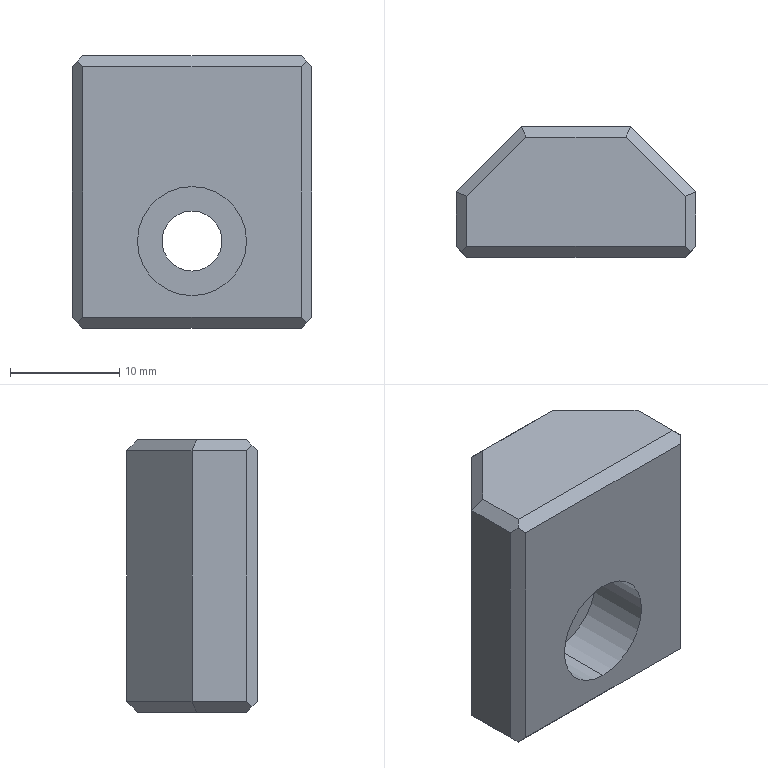Part | Creo | 1 solid | 27 faces | box 22 x 12 x 25 mm | volume 5004 mm3 | plane 23 | cylinder 4 | commonest cylinder face diameters 5.5 x2 10 x2
STEP:
#1=CARTESIAN_POINT('',(34.742,-375.005,-60.5));
#2=VERTEX_POINT('',#1);
#3=CARTESIAN_POINT('',(34.742,-375.005,-70.5));
#4=VERTEX_POINT('',#3);
#5=CARTESIAN_POINT('',(34.742,-375.005,-65.5));
#6=DIRECTION('',(0.,1.,0.));
#7=DIRECTION('',(0.,0.,1.));
#8=AXIS2_PLACEMENT_3D('',#5,#6,#7);
#9=CIRCLE('',#8,5.);
#10=EDGE_CURVE('',#2,#4,#9,.T.);
#11=ORIENTED_EDGE('',*,*,#10,.T.);
#12=CARTESIAN_POINT('',(34.742,-369.005,-70.5));
#13=VERTEX_POINT('',#12);
#14=CARTESIAN_POINT('',(34.742,-375.005,-70.5));
#15=DIRECTION('',(0.,1.,0.));
#16=VECTOR('',#15,6.);
#17=LINE('',#14,#16);
#18=EDGE_CURVE('',#4,#13,#17,.T.);
#19=ORIENTED_EDGE('',*,*,#18,.T.);
#20=CARTESIAN_POINT('',(34.742,-369.005,-60.5));
#21=VERTEX_POINT('',#20);
#22=CARTESIAN_POINT('',(34.742,-369.005,-65.5));
#23=DIRECTION('',(0.,-1.,0.));
#24=DIRECTION('',(0.,0.,-1.));
#25=AXIS2_PLACEMENT_3D('',#22,#23,#24);
#26=CIRCLE('',#25,5.);
#27=EDGE_CURVE('',#13,#21,#26,.T.);
#28=ORIENTED_EDGE('',*,*,#27,.T.);
#29=CARTESIAN_POINT('',(34.742,-375.005,-60.5));
#30=DIRECTION('',(0.,1.,0.));
#31=VECTOR('',#30,6.);
#32=LINE('',#29,#31);
#33=EDGE_CURVE('',#2,#21,#32,.T.);
#34=ORIENTED_EDGE('',*,*,#33,.F.);
#35=EDGE_LOOP('',(#11,#19,#28,#34));
#36=FACE_OUTER_BOUND('',#35,.F.);
#37=CARTESIAN_POINT('',(34.742,-375.305,-65.5));
#38=DIRECTION('',(0.,1.,0.));
#39=DIRECTION('',(0.,0.,1.));
#40=AXIS2_PLACEMENT_3D('',#37,#38,#39);
#41=CYLINDRICAL_SURFACE('',#40,5.);
#42=ADVANCED_FACE('',(#36),#41,.F.);
#43=CARTESIAN_POINT('',(44.742,-375.005,-72.5));
#44=VERTEX_POINT('',#43);
#45=CARTESIAN_POINT('',(44.742,-375.005,-49.5));
#46=VERTEX_POINT('',#45);
#47=CARTESIAN_POINT('',(44.742,-375.005,-72.5));
#48=DIRECTION('',(0.,0.,1.));
#49=VECTOR('',#48,23.);
#50=LINE('',#47,#49);
#51=EDGE_CURVE('',#44,#46,#50,.T.);
#52=ORIENTED_EDGE('',*,*,#51,.F.);
#53=CARTESIAN_POINT('',(24.742,-375.005,-72.5));
#54=VERTEX_POINT('',#53);
#55=CARTESIAN_POINT('',(44.742,-375.005,-72.5));
#56=DIRECTION('',(-1.,0.,0.));
#57=VECTOR('',#56,20.);
#58=LINE('',#55,#57);
#59=EDGE_CURVE('',#44,#54,#58,.T.);
#60=ORIENTED_EDGE('',*,*,#59,.T.);
#61=CARTESIAN_POINT('',(24.742,-375.005,-49.5));
#62=VERTEX_POINT('',#61);
#63=CARTESIAN_POINT('',(24.742,-375.005,-49.5));
#64=DIRECTION('',(0.,0.,-1.));
#65=VECTOR('',#64,23.);
#66=LINE('',#63,#65);
#67=EDGE_CURVE('',#62,#54,#66,.T.);
#68=ORIENTED_EDGE('',*,*,#67,.F.);
#69=CARTESIAN_POINT('',(44.742,-375.005,-49.5));
#70=DIRECTION('',(-1.,0.,0.));
#71=VECTOR('',#70,20.);
#72=LINE('',#69,#71);
#73=EDGE_CURVE('',#46,#62,#72,.T.);
#74=ORIENTED_EDGE('',*,*,#73,.F.);
#75=EDGE_LOOP('',(#52,#60,#68,#74));
#76=FACE_OUTER_BOUND('',#75,.F.);
#77=CARTESIAN_POINT('',(34.742,-375.005,-65.5));
#78=DIRECTION('',(0.,1.,0.));
#79=DIRECTION('',(0.,0.,-1.));
#80=AXIS2_PLACEMENT_3D('',#77,#78,#79);
#81=CIRCLE('',#80,5.);
#82=EDGE_CURVE('',#4,#2,#81,.T.);
#83=ORIENTED_EDGE('',*,*,#82,.F.);
#84=ORIENTED_EDGE('',*,*,#10,.F.);
#85=EDGE_LOOP('',(#83,#84));
#86=FACE_BOUND('',#85,.F.);
#87=CARTESIAN_POINT('',(45.742,-375.005,-73.5));
#88=DIRECTION('',(0.,-1.,0.));
#89=DIRECTION('',(0.,0.,-1.));
#90=AXIS2_PLACEMENT_3D('',#87,#88,#89);
#91=PLANE('',#90);
#92=ADVANCED_FACE('',(#76,#86),#91,.T.);
#93=ORIENTED_EDGE('',*,*,#82,.T.);
#94=ORIENTED_EDGE('',*,*,#33,.T.);
#95=CARTESIAN_POINT('',(34.742,-369.005,-65.5));
#96=DIRECTION('',(0.,-1.,0.));
#97=DIRECTION('',(0.,0.,1.));
#98=AXIS2_PLACEMENT_3D('',#95,#96,#97);
#99=CIRCLE('',#98,5.);
#100=EDGE_CURVE('',#21,#13,#99,.T.);
#101=ORIENTED_EDGE('',*,*,#100,.T.);
#102=ORIENTED_EDGE('',*,*,#18,.F.);
#103=EDGE_LOOP('',(#93,#94,#101,#102));
#104=FACE_OUTER_BOUND('',#103,.F.);
#105=CARTESIAN_POINT('',(34.742,-375.305,-65.5));
#106=DIRECTION('',(0.,1.,0.));
#107=DIRECTION('',(0.,0.,1.));
#108=AXIS2_PLACEMENT_3D('',#105,#106,#107);
#109=CYLINDRICAL_SURFACE('',#108,5.);
#110=ADVANCED_FACE('',(#104),#109,.F.);
#111=ORIENTED_EDGE('',*,*,#27,.F.);
#112=ORIENTED_EDGE('',*,*,#100,.F.);
#113=EDGE_LOOP('',(#111,#112));
#114=FACE_OUTER_BOUND('',#113,.F.);
#115=CARTESIAN_POINT('',(34.742,-369.005,-68.25));
#116=VERTEX_POINT('',#115);
#117=CARTESIAN_POINT('',(34.742,-369.005,-62.75));
#118=VERTEX_POINT('',#117);
#119=CARTESIAN_POINT('',(34.742,-369.005,-65.5));
#120=DIRECTION('',(0.,1.,0.));
#121=DIRECTION('',(0.,0.,-1.));
#122=AXIS2_PLACEMENT_3D('',#119,#120,#121);
#123=CIRCLE('',#122,2.75);
#124=EDGE_CURVE('',#116,#118,#123,.T.);
#125=ORIENTED_EDGE('',*,*,#124,.F.);
#126=CARTESIAN_POINT('',(34.742,-369.005,-65.5));
#127=DIRECTION('',(0.,1.,0.));
#128=DIRECTION('',(0.,0.,1.));
#129=AXIS2_PLACEMENT_3D('',#126,#127,#128);
#130=CIRCLE('',#129,2.75);
#131=EDGE_CURVE('',#118,#116,#130,.T.);
#132=ORIENTED_EDGE('',*,*,#131,.F.);
#133=EDGE_LOOP('',(#125,#132));
#134=FACE_BOUND('',#133,.F.);
#135=CARTESIAN_POINT('',(34.742,-369.005,-65.5));
#136=DIRECTION('',(0.,1.,0.));
#137=DIRECTION('',(0.,0.,1.));
#138=AXIS2_PLACEMENT_3D('',#135,#136,#137);
#139=PLANE('',#138);
#140=ADVANCED_FACE('',(#114,#134),#139,.F.);
#141=CARTESIAN_POINT('',(34.742,-363.005,-62.75));
#142=VERTEX_POINT('',#141);
#143=CARTESIAN_POINT('',(34.742,-363.005,-68.25));
#144=VERTEX_POINT('',#143);
#145=CARTESIAN_POINT('',(34.742,-363.005,-65.5));
#146=DIRECTION('',(0.,-1.,0.));
#147=DIRECTION('',(0.,0.,1.));
#148=AXIS2_PLACEMENT_3D('',#145,#146,#147);
#149=CIRCLE('',#148,2.75);
#150=EDGE_CURVE('',#142,#144,#149,.T.);
#151=ORIENTED_EDGE('',*,*,#150,.T.);
#152=CARTESIAN_POINT('',(34.742,-363.005,-68.25));
#153=DIRECTION('',(0.,-1.,0.));
#154=VECTOR('',#153,6.);
#155=LINE('',#152,#154);
#156=EDGE_CURVE('',#144,#116,#155,.T.);
#157=ORIENTED_EDGE('',*,*,#156,.T.);
#158=ORIENTED_EDGE('',*,*,#124,.T.);
#159=CARTESIAN_POINT('',(34.742,-363.005,-62.75));
#160=DIRECTION('',(0.,-1.,0.));
#161=VECTOR('',#160,6.);
#162=LINE('',#159,#161);
#163=EDGE_CURVE('',#142,#118,#162,.T.);
#164=ORIENTED_EDGE('',*,*,#163,.F.);
#165=EDGE_LOOP('',(#151,#157,#158,#164));
#166=FACE_OUTER_BOUND('',#165,.F.);
#167=CARTESIAN_POINT('',(34.742,-369.005,-65.5));
#168=DIRECTION('',(0.,-1.,0.));
#169=DIRECTION('',(0.,0.,1.));
#170=AXIS2_PLACEMENT_3D('',#167,#168,#169);
#171=CYLINDRICAL_SURFACE('',#170,2.75);
#172=ADVANCED_FACE('',(#166),#171,.F.);
#173=CARTESIAN_POINT('',(29.742,-363.005,-72.5));
#174=VERTEX_POINT('',#173);
#175=CARTESIAN_POINT('',(29.742,-363.005,-49.5));
#176=VERTEX_POINT('',#175);
#177=CARTESIAN_POINT('',(29.742,-363.005,-72.5));
#178=DIRECTION('',(0.,0.,1.));
#179=VECTOR('',#178,23.);
#180=LINE('',#177,#179);
#181=EDGE_CURVE('',#174,#176,#180,.T.);
#182=ORIENTED_EDGE('',*,*,#181,.F.);
#183=CARTESIAN_POINT('',(39.742,-363.005,-72.5));
#184=VERTEX_POINT('',#183);
#185=CARTESIAN_POINT('',(39.742,-363.005,-72.5));
#186=DIRECTION('',(-1.,0.,0.));
#187=VECTOR('',#186,10.);
#188=LINE('',#185,#187);
#189=EDGE_CURVE('',#184,#174,#188,.T.);
#190=ORIENTED_EDGE('',*,*,#189,.F.);
#191=CARTESIAN_POINT('',(39.742,-363.005,-49.5));
#192=VERTEX_POINT('',#191);
#193=CARTESIAN_POINT('',(39.742,-363.005,-49.5));
#194=DIRECTION('',(0.,0.,-1.));
#195=VECTOR('',#194,23.);
#196=LINE('',#193,#195);
#197=EDGE_CURVE('',#192,#184,#196,.T.);
#198=ORIENTED_EDGE('',*,*,#197,.F.);
#199=CARTESIAN_POINT('',(39.742,-363.005,-49.5));
#200=DIRECTION('',(-1.,0.,0.));
#201=VECTOR('',#200,10.);
#202=LINE('',#199,#201);
#203=EDGE_CURVE('',#192,#176,#202,.T.);
#204=ORIENTED_EDGE('',*,*,#203,.T.);
#205=EDGE_LOOP('',(#182,#190,#198,#204));
#206=FACE_OUTER_BOUND('',#205,.F.);
#207=CARTESIAN_POINT('',(34.742,-363.005,-65.5));
#208=DIRECTION('',(0.,-1.,0.));
#209=DIRECTION('',(0.,0.,-1.));
#210=AXIS2_PLACEMENT_3D('',#207,#208,#209);
#211=CIRCLE('',#210,2.75);
#212=EDGE_CURVE('',#144,#142,#211,.T.);
#213=ORIENTED_EDGE('',*,*,#212,.F.);
#214=ORIENTED_EDGE('',*,*,#150,.F.);
#215=EDGE_LOOP('',(#213,#214));
#216=FACE_BOUND('',#215,.F.);
#217=CARTESIAN_POINT('',(45.742,-363.005,-48.5));
#218=DIRECTION('',(0.,1.,0.));
#219=DIRECTION('',(0.,0.,1.));
#220=AXIS2_PLACEMENT_3D('',#217,#218,#219);
#221=PLANE('',#220);
#222=ADVANCED_FACE('',(#206,#216),#221,.T.);
#223=ORIENTED_EDGE('',*,*,#212,.T.);
#224=ORIENTED_EDGE('',*,*,#163,.T.);
#225=ORIENTED_EDGE('',*,*,#131,.T.);
#226=ORIENTED_EDGE('',*,*,#156,.F.);
#227=EDGE_LOOP('',(#223,#224,#225,#226));
#228=FACE_OUTER_BOUND('',#227,.F.);
#229=CARTESIAN_POINT('',(34.742,-369.005,-65.5));
#230=DIRECTION('',(0.,-1.,0.));
#231=DIRECTION('',(0.,0.,1.));
#232=AXIS2_PLACEMENT_3D('',#229,#230,#231);
#233=CYLINDRICAL_SURFACE('',#232,2.75);
#234=ADVANCED_FACE('',(#228),#233,.F.);
#235=CARTESIAN_POINT('',(23.742,-369.005,-72.5));
#236=VERTEX_POINT('',#235);
#237=CARTESIAN_POINT('',(23.742,-369.005,-49.5));
#238=VERTEX_POINT('',#237);
#239=CARTESIAN_POINT('',(23.742,-369.005,-72.5));
#240=DIRECTION('',(0.,0.,1.));
#241=VECTOR('',#240,23.);
#242=LINE('',#239,#241);
#243=EDGE_CURVE('',#236,#238,#242,.T.);
#244=ORIENTED_EDGE('',*,*,#243,.F.);
#245=CARTESIAN_POINT('',(29.742,-363.005,-72.5));
#246=DIRECTION('',(-0.7071,-0.7071,0.));
#247=VECTOR('',#246,8.485);
#248=LINE('',#245,#247);
#249=EDGE_CURVE('',#174,#236,#248,.T.);
#250=ORIENTED_EDGE('',*,*,#249,.F.);
#251=ORIENTED_EDGE('',*,*,#181,.T.);
#252=CARTESIAN_POINT('',(23.742,-369.005,-49.5));
#253=DIRECTION('',(0.7071,0.7071,0.));
#254=VECTOR('',#253,8.485);
#255=LINE('',#252,#254);
#256=EDGE_CURVE('',#238,#176,#255,.T.);
#257=ORIENTED_EDGE('',*,*,#256,.F.);
#258=EDGE_LOOP('',(#244,#250,#251,#257));
#259=FACE_OUTER_BOUND('',#258,.F.);
#260=CARTESIAN_POINT('',(26.742,-366.005,-61.));
#261=DIRECTION('',(-0.7071,0.7071,0.));
#262=DIRECTION('',(0.,0.,1.));
#263=AXIS2_PLACEMENT_3D('',#260,#261,#262);
#264=PLANE('',#263);
#265=ADVANCED_FACE('',(#259),#264,.T.);
#266=CARTESIAN_POINT('',(23.742,-374.005,-49.5));
#267=VERTEX_POINT('',#266);
#268=CARTESIAN_POINT('',(23.742,-374.005,-72.5));
#269=VERTEX_POINT('',#268);
#270=CARTESIAN_POINT('',(23.742,-374.005,-49.5));
#271=DIRECTION('',(0.,0.,-1.));
#272=VECTOR('',#271,23.);
#273=LINE('',#270,#272);
#274=EDGE_CURVE('',#267,#269,#273,.T.);
#275=ORIENTED_EDGE('',*,*,#274,.T.);
#276=CARTESIAN_POINT('',(23.742,-374.005,-72.5));
#277=DIRECTION('',(0.,1.,0.));
#278=VECTOR('',#277,5.);
#279=LINE('',#276,#278);
#280=EDGE_CURVE('',#269,#236,#279,.T.);
#281=ORIENTED_EDGE('',*,*,#280,.T.);
#282=ORIENTED_EDGE('',*,*,#243,.T.);
#283=CARTESIAN_POINT('',(23.742,-369.005,-49.5));
#284=DIRECTION('',(0.,-1.,0.));
#285=VECTOR('',#284,5.);
#286=LINE('',#283,#285);
#287=EDGE_CURVE('',#238,#267,#286,.T.);
#288=ORIENTED_EDGE('',*,*,#287,.T.);
#289=EDGE_LOOP('',(#275,#281,#282,#288));
#290=FACE_OUTER_BOUND('',#289,.F.);
#291=CARTESIAN_POINT('',(23.742,-375.005,-53.5));
#292=DIRECTION('',(-1.,0.,0.));
#293=DIRECTION('',(0.,1.,0.));
#294=AXIS2_PLACEMENT_3D('',#291,#292,#293);
#295=PLANE('',#294);
#296=ADVANCED_FACE('',(#290),#295,.T.);
#297=CARTESIAN_POINT('',(24.242,-374.505,-49.));
#298=VERTEX_POINT('',#297);
#299=CARTESIAN_POINT('',(24.742,-375.005,-49.5));
#300=DIRECTION('',(-0.5774,0.5774,0.5774));
#301=VECTOR('',#300,0.866);
#302=LINE('',#299,#301);
#303=EDGE_CURVE('',#62,#298,#302,.T.);
#304=ORIENTED_EDGE('',*,*,#303,.F.);
#305=ORIENTED_EDGE('',*,*,#67,.T.);
#306=CARTESIAN_POINT('',(24.242,-374.505,-73.));
#307=VERTEX_POINT('',#306);
#308=CARTESIAN_POINT('',(24.242,-374.505,-73.));
#309=DIRECTION('',(0.5774,-0.5774,0.5774));
#310=VECTOR('',#309,0.866);
#311=LINE('',#308,#310);
#312=EDGE_CURVE('',#307,#54,#311,.T.);
#313=ORIENTED_EDGE('',*,*,#312,.F.);
#314=CARTESIAN_POINT('',(23.742,-374.005,-72.5));
#315=DIRECTION('',(0.5774,-0.5774,-0.5774));
#316=VECTOR('',#315,0.866);
#317=LINE('',#314,#316);
#318=EDGE_CURVE('',#269,#307,#317,.T.);
#319=ORIENTED_EDGE('',*,*,#318,.F.);
#320=ORIENTED_EDGE('',*,*,#274,.F.);
#321=CARTESIAN_POINT('',(24.242,-374.505,-49.));
#322=DIRECTION('',(-0.5774,0.5774,-0.5774));
#323=VECTOR('',#322,0.866);
#324=LINE('',#321,#323);
#325=EDGE_CURVE('',#298,#267,#324,.T.);
#326=ORIENTED_EDGE('',*,*,#325,.F.);
#327=EDGE_LOOP('',(#304,#305,#313,#319,#320,#326));
#328=FACE_OUTER_BOUND('',#327,.F.);
#329=CARTESIAN_POINT('',(24.242,-374.505,-61.));
#330=DIRECTION('',(-0.7071,-0.7071,0.));
#331=DIRECTION('',(-0.7071,0.7071,0.));
#332=AXIS2_PLACEMENT_3D('',#329,#330,#331);
#333=PLANE('',#332);
#334=ADVANCED_FACE('',(#328),#333,.T.);
#335=CARTESIAN_POINT('',(24.742,-374.005,-48.5));
#336=VERTEX_POINT('',#335);
#337=CARTESIAN_POINT('',(24.242,-374.505,-49.));
#338=DIRECTION('',(0.5774,0.5774,0.5774));
#339=VECTOR('',#338,0.866);
#340=LINE('',#337,#339);
#341=EDGE_CURVE('',#298,#336,#340,.T.);
#342=ORIENTED_EDGE('',*,*,#341,.T.);
#343=CARTESIAN_POINT('',(44.742,-374.005,-48.5));
#344=VERTEX_POINT('',#343);
#345=CARTESIAN_POINT('',(44.742,-374.005,-48.5));
#346=DIRECTION('',(-1.,0.,0.));
#347=VECTOR('',#346,20.);
#348=LINE('',#345,#347);
#349=EDGE_CURVE('',#344,#336,#348,.T.);
#350=ORIENTED_EDGE('',*,*,#349,.F.);
#351=CARTESIAN_POINT('',(45.242,-374.505,-49.));
#352=VERTEX_POINT('',#351);
#353=CARTESIAN_POINT('',(45.242,-374.505,-49.));
#354=DIRECTION('',(-0.5774,0.5774,0.5774));
#355=VECTOR('',#354,0.866);
#356=LINE('',#353,#355);
#357=EDGE_CURVE('',#352,#344,#356,.T.);
#358=ORIENTED_EDGE('',*,*,#357,.F.);
#359=CARTESIAN_POINT('',(45.242,-374.505,-49.));
#360=DIRECTION('',(-0.5774,-0.5774,-0.5774));
#361=VECTOR('',#360,0.866);
#362=LINE('',#359,#361);
#363=EDGE_CURVE('',#352,#46,#362,.T.);
#364=ORIENTED_EDGE('',*,*,#363,.T.);
#365=ORIENTED_EDGE('',*,*,#73,.T.);
#366=ORIENTED_EDGE('',*,*,#303,.T.);
#367=EDGE_LOOP('',(#342,#350,#358,#364,#365,#366));
#368=FACE_OUTER_BOUND('',#367,.F.);
#369=CARTESIAN_POINT('',(34.742,-374.505,-49.));
#370=DIRECTION('',(0.,-0.7071,0.7071));
#371=DIRECTION('',(0.,0.7071,0.7071));
#372=AXIS2_PLACEMENT_3D('',#369,#370,#371);
#373=PLANE('',#372);
#374=ADVANCED_FACE('',(#368),#373,.T.);
#375=CARTESIAN_POINT('',(24.742,-369.419,-48.5));
#376=VERTEX_POINT('',#375);
#377=CARTESIAN_POINT('',(24.742,-369.419,-48.5));
#378=DIRECTION('',(-0.6786,0.2811,-0.6786));
#379=VECTOR('',#378,1.474);
#380=LINE('',#377,#379);
#381=EDGE_CURVE('',#376,#238,#380,.T.);
#382=ORIENTED_EDGE('',*,*,#381,.F.);
#383=CARTESIAN_POINT('',(24.742,-369.419,-48.5));
#384=DIRECTION('',(0.,-1.,0.));
#385=VECTOR('',#384,4.586);
#386=LINE('',#383,#385);
#387=EDGE_CURVE('',#376,#336,#386,.T.);
#388=ORIENTED_EDGE('',*,*,#387,.T.);
#389=ORIENTED_EDGE('',*,*,#341,.F.);
#390=ORIENTED_EDGE('',*,*,#325,.T.);
#391=ORIENTED_EDGE('',*,*,#287,.F.);
#392=EDGE_LOOP('',(#382,#388,#389,#390,#391));
#393=FACE_OUTER_BOUND('',#392,.F.);
#394=CARTESIAN_POINT('',(24.242,-372.005,-49.));
#395=DIRECTION('',(-0.7071,0.,0.7071));
#396=DIRECTION('',(-0.7071,0.,-0.7071));
#397=AXIS2_PLACEMENT_3D('',#394,#395,#396);
#398=PLANE('',#397);
#399=ADVANCED_FACE('',(#393),#398,.T.);
#400=CARTESIAN_POINT('',(30.156,-364.005,-48.5));
#401=VERTEX_POINT('',#400);
#402=CARTESIAN_POINT('',(30.156,-364.005,-48.5));
#403=DIRECTION('',(-0.2811,0.6786,-0.6786));
#404=VECTOR('',#403,1.474);
#405=LINE('',#402,#404);
#406=EDGE_CURVE('',#401,#176,#405,.T.);
#407=ORIENTED_EDGE('',*,*,#406,.F.);
#408=CARTESIAN_POINT('',(30.156,-364.005,-48.5));
#409=DIRECTION('',(-0.7071,-0.7071,0.));
#410=VECTOR('',#409,7.657);
#411=LINE('',#408,#410);
#412=EDGE_CURVE('',#401,#376,#411,.T.);
#413=ORIENTED_EDGE('',*,*,#412,.T.);
#414=ORIENTED_EDGE('',*,*,#381,.T.);
#415=ORIENTED_EDGE('',*,*,#256,.T.);
#416=EDGE_LOOP('',(#407,#413,#414,#415));
#417=FACE_OUTER_BOUND('',#416,.F.);
#418=CARTESIAN_POINT('',(27.095,-366.358,-49.));
#419=DIRECTION('',(-0.5,0.5,0.7071));
#420=DIRECTION('',(0.5,-0.5,0.7071));
#421=AXIS2_PLACEMENT_3D('',#418,#419,#420);
#422=PLANE('',#421);
#423=ADVANCED_FACE('',(#417),#422,.T.);
#424=CARTESIAN_POINT('',(39.327,-364.005,-48.5));
#425=VERTEX_POINT('',#424);
#426=CARTESIAN_POINT('',(39.327,-364.005,-48.5));
#427=DIRECTION('',(0.2811,0.6786,-0.6786));
#428=VECTOR('',#427,1.474);
#429=LINE('',#426,#428);
#430=EDGE_CURVE('',#425,#192,#429,.T.);
#431=ORIENTED_EDGE('',*,*,#430,.F.);
#432=CARTESIAN_POINT('',(39.327,-364.005,-48.5));
#433=DIRECTION('',(-1.,0.,0.));
#434=VECTOR('',#433,9.172);
#435=LINE('',#432,#434);
#436=EDGE_CURVE('',#425,#401,#435,.T.);
#437=ORIENTED_EDGE('',*,*,#436,.T.);
#438=ORIENTED_EDGE('',*,*,#406,.T.);
#439=ORIENTED_EDGE('',*,*,#203,.F.);
#440=EDGE_LOOP('',(#431,#437,#438,#439));
#441=FACE_OUTER_BOUND('',#440,.F.);
#442=CARTESIAN_POINT('',(34.742,-363.505,-49.));
#443=DIRECTION('',(0.,0.7071,0.7071));
#444=DIRECTION('',(0.,0.7071,-0.7071));
#445=AXIS2_PLACEMENT_3D('',#442,#443,#444);
#446=PLANE('',#445);
#447=ADVANCED_FACE('',(#441),#446,.T.);
#448=ORIENTED_EDGE('',*,*,#430,.T.);
#449=CARTESIAN_POINT('',(45.742,-369.005,-49.5));
#450=VERTEX_POINT('',#449);
#451=CARTESIAN_POINT('',(39.742,-363.005,-49.5));
#452=DIRECTION('',(0.7071,-0.7071,0.));
#453=VECTOR('',#452,8.485);
#454=LINE('',#451,#453);
#455=EDGE_CURVE('',#192,#450,#454,.T.);
#456=ORIENTED_EDGE('',*,*,#455,.T.);
#457=CARTESIAN_POINT('',(44.742,-369.419,-48.5));
#458=VERTEX_POINT('',#457);
#459=CARTESIAN_POINT('',(45.742,-369.005,-49.5));
#460=DIRECTION('',(-0.6786,-0.2811,0.6786));
#461=VECTOR('',#460,1.474);
#462=LINE('',#459,#461);
#463=EDGE_CURVE('',#450,#458,#462,.T.);
#464=ORIENTED_EDGE('',*,*,#463,.T.);
#465=CARTESIAN_POINT('',(44.742,-369.419,-48.5));
#466=DIRECTION('',(-0.7071,0.7071,0.));
#467=VECTOR('',#466,7.657);
#468=LINE('',#465,#467);
#469=EDGE_CURVE('',#458,#425,#468,.T.);
#470=ORIENTED_EDGE('',*,*,#469,.T.);
#471=EDGE_LOOP('',(#448,#456,#464,#470));
#472=FACE_OUTER_BOUND('',#471,.F.);
#473=CARTESIAN_POINT('',(42.388,-366.358,-49.));
#474=DIRECTION('',(0.5,0.5,0.7071));
#475=DIRECTION('',(-0.5,-0.5,0.7071));
#476=AXIS2_PLACEMENT_3D('',#473,#474,#475);
#477=PLANE('',#476);
#478=ADVANCED_FACE('',(#472),#477,.T.);
#479=ORIENTED_EDGE('',*,*,#197,.T.);
#480=CARTESIAN_POINT('',(45.742,-369.005,-72.5));
#481=VERTEX_POINT('',#480);
#482=CARTESIAN_POINT('',(45.742,-369.005,-72.5));
#483=DIRECTION('',(-0.7071,0.7071,0.));
#484=VECTOR('',#483,8.485);
#485=LINE('',#482,#484);
#486=EDGE_CURVE('',#481,#184,#485,.T.);
#487=ORIENTED_EDGE('',*,*,#486,.F.);
#488=CARTESIAN_POINT('',(45.742,-369.005,-49.5));
#489=DIRECTION('',(0.,0.,-1.));
#490=VECTOR('',#489,23.);
#491=LINE('',#488,#490);
#492=EDGE_CURVE('',#450,#481,#491,.T.);
#493=ORIENTED_EDGE('',*,*,#492,.F.);
#494=ORIENTED_EDGE('',*,*,#455,.F.);
#495=EDGE_LOOP('',(#479,#487,#493,#494));
#496=FACE_OUTER_BOUND('',#495,.F.);
#497=CARTESIAN_POINT('',(42.742,-366.005,-61.));
#498=DIRECTION('',(0.7071,0.7071,0.));
#499=DIRECTION('',(0.,0.,1.));
#500=AXIS2_PLACEMENT_3D('',#497,#498,#499);
#501=PLANE('',#500);
#502=ADVANCED_FACE('',(#496),#501,.T.);
#503=CARTESIAN_POINT('',(44.742,-369.419,-73.5));
#504=VERTEX_POINT('',#503);
#505=CARTESIAN_POINT('',(45.742,-369.005,-72.5));
#506=DIRECTION('',(-0.6786,-0.2811,-0.6786));
#507=VECTOR('',#506,1.474);
#508=LINE('',#505,#507);
#509=EDGE_CURVE('',#481,#504,#508,.T.);
#510=ORIENTED_EDGE('',*,*,#509,.F.);
#511=ORIENTED_EDGE('',*,*,#486,.T.);
#512=CARTESIAN_POINT('',(39.327,-364.005,-73.5));
#513=VERTEX_POINT('',#512);
#514=CARTESIAN_POINT('',(39.742,-363.005,-72.5));
#515=DIRECTION('',(-0.2811,-0.6786,-0.6786));
#516=VECTOR('',#515,1.474);
#517=LINE('',#514,#516);
#518=EDGE_CURVE('',#184,#513,#517,.T.);
#519=ORIENTED_EDGE('',*,*,#518,.T.);
#520=CARTESIAN_POINT('',(39.327,-364.005,-73.5));
#521=DIRECTION('',(0.7071,-0.7071,0.));
#522=VECTOR('',#521,7.657);
#523=LINE('',#520,#522);
#524=EDGE_CURVE('',#513,#504,#523,.T.);
#525=ORIENTED_EDGE('',*,*,#524,.T.);
#526=EDGE_LOOP('',(#510,#511,#519,#525));
#527=FACE_OUTER_BOUND('',#526,.F.);
#528=CARTESIAN_POINT('',(42.388,-366.358,-73.));
#529=DIRECTION('',(0.5,0.5,-0.7071));
#530=DIRECTION('',(-0.5,-0.5,-0.7071));
#531=AXIS2_PLACEMENT_3D('',#528,#529,#530);
#532=PLANE('',#531);
#533=ADVANCED_FACE('',(#527),#532,.T.);
#534=ORIENTED_EDGE('',*,*,#509,.T.);
#535=CARTESIAN_POINT('',(44.742,-374.005,-73.5));
#536=VERTEX_POINT('',#535);
#537=CARTESIAN_POINT('',(44.742,-369.419,-73.5));
#538=DIRECTION('',(0.,-1.,0.));
#539=VECTOR('',#538,4.586);
#540=LINE('',#537,#539);
#541=EDGE_CURVE('',#504,#536,#540,.T.);
#542=ORIENTED_EDGE('',*,*,#541,.T.);
#543=CARTESIAN_POINT('',(45.242,-374.505,-73.));
#544=VERTEX_POINT('',#543);
#545=CARTESIAN_POINT('',(45.242,-374.505,-73.));
#546=DIRECTION('',(-0.5774,0.5774,-0.5774));
#547=VECTOR('',#546,0.866);
#548=LINE('',#545,#547);
#549=EDGE_CURVE('',#544,#536,#548,.T.);
#550=ORIENTED_EDGE('',*,*,#549,.F.);
#551=CARTESIAN_POINT('',(45.742,-374.005,-72.5));
#552=VERTEX_POINT('',#551);
#553=CARTESIAN_POINT('',(45.242,-374.505,-73.));
#554=DIRECTION('',(0.5774,0.5774,0.5774));
#555=VECTOR('',#554,0.866);
#556=LINE('',#553,#555);
#557=EDGE_CURVE('',#544,#552,#556,.T.);
#558=ORIENTED_EDGE('',*,*,#557,.T.);
#559=CARTESIAN_POINT('',(45.742,-369.005,-72.5));
#560=DIRECTION('',(0.,-1.,0.));
#561=VECTOR('',#560,5.);
#562=LINE('',#559,#561);
#563=EDGE_CURVE('',#481,#552,#562,.T.);
#564=ORIENTED_EDGE('',*,*,#563,.F.);
#565=EDGE_LOOP('',(#534,#542,#550,#558,#564));
#566=FACE_OUTER_BOUND('',#565,.F.);
#567=CARTESIAN_POINT('',(45.242,-372.005,-73.));
#568=DIRECTION('',(0.7071,0.,-0.7071));
#569=DIRECTION('',(0.7071,0.,0.7071));
#570=AXIS2_PLACEMENT_3D('',#567,#568,#569);
#571=PLANE('',#570);
#572=ADVANCED_FACE('',(#566),#571,.T.);
#573=CARTESIAN_POINT('',(24.742,-374.005,-73.5));
#574=VERTEX_POINT('',#573);
#575=CARTESIAN_POINT('',(24.742,-369.419,-73.5));
#576=VERTEX_POINT('',#575);
#577=CARTESIAN_POINT('',(24.742,-374.005,-73.5));
#578=DIRECTION('',(0.,1.,0.));
#579=VECTOR('',#578,4.586);
#580=LINE('',#577,#579);
#581=EDGE_CURVE('',#574,#576,#580,.T.);
#582=ORIENTED_EDGE('',*,*,#581,.F.);
#583=CARTESIAN_POINT('',(44.742,-374.005,-73.5));
#584=DIRECTION('',(-1.,0.,0.));
#585=VECTOR('',#584,20.);
#586=LINE('',#583,#585);
#587=EDGE_CURVE('',#536,#574,#586,.T.);
#588=ORIENTED_EDGE('',*,*,#587,.F.);
#589=ORIENTED_EDGE('',*,*,#541,.F.);
#590=ORIENTED_EDGE('',*,*,#524,.F.);
#591=CARTESIAN_POINT('',(30.156,-364.005,-73.5));
#592=VERTEX_POINT('',#591);
#593=CARTESIAN_POINT('',(39.327,-364.005,-73.5));
#594=DIRECTION('',(-1.,0.,0.));
#595=VECTOR('',#594,9.172);
#596=LINE('',#593,#595);
#597=EDGE_CURVE('',#513,#592,#596,.T.);
#598=ORIENTED_EDGE('',*,*,#597,.T.);
#599=CARTESIAN_POINT('',(24.742,-369.419,-73.5));
#600=DIRECTION('',(0.7071,0.7071,0.));
#601=VECTOR('',#600,7.657);
#602=LINE('',#599,#601);
#603=EDGE_CURVE('',#576,#592,#602,.T.);
#604=ORIENTED_EDGE('',*,*,#603,.F.);
#605=EDGE_LOOP('',(#582,#588,#589,#590,#598,#604));
#606=FACE_OUTER_BOUND('',#605,.F.);
#607=CARTESIAN_POINT('',(45.742,-363.005,-73.5));
#608=DIRECTION('',(0.,0.,-1.));
#609=DIRECTION('',(0.,1.,0.));
#610=AXIS2_PLACEMENT_3D('',#607,#608,#609);
#611=PLANE('',#610);
#612=ADVANCED_FACE('',(#606),#611,.T.);
#613=CARTESIAN_POINT('',(23.742,-369.005,-72.5));
#614=DIRECTION('',(0.6786,-0.2811,-0.6786));
#615=VECTOR('',#614,1.474);
#616=LINE('',#613,#615);
#617=EDGE_CURVE('',#236,#576,#616,.T.);
#618=ORIENTED_EDGE('',*,*,#617,.F.);
#619=ORIENTED_EDGE('',*,*,#280,.F.);
#620=ORIENTED_EDGE('',*,*,#318,.T.);
#621=CARTESIAN_POINT('',(24.242,-374.505,-73.));
#622=DIRECTION('',(0.5774,0.5774,-0.5774));
#623=VECTOR('',#622,0.866);
#624=LINE('',#621,#623);
#625=EDGE_CURVE('',#307,#574,#624,.T.);
#626=ORIENTED_EDGE('',*,*,#625,.T.);
#627=ORIENTED_EDGE('',*,*,#581,.T.);
#628=EDGE_LOOP('',(#618,#619,#620,#626,#627));
#629=FACE_OUTER_BOUND('',#628,.F.);
#630=CARTESIAN_POINT('',(24.242,-372.005,-73.));
#631=DIRECTION('',(-0.7071,0.,-0.7071));
#632=DIRECTION('',(-0.7071,0.,0.7071));
#633=AXIS2_PLACEMENT_3D('',#630,#631,#632);
#634=PLANE('',#633);
#635=ADVANCED_FACE('',(#629),#634,.T.);
#636=ORIENTED_EDGE('',*,*,#617,.T.);
#637=ORIENTED_EDGE('',*,*,#603,.T.);
#638=CARTESIAN_POINT('',(29.742,-363.005,-72.5));
#639=DIRECTION('',(0.2811,-0.6786,-0.6786));
#640=VECTOR('',#639,1.474);
#641=LINE('',#638,#640);
#642=EDGE_CURVE('',#174,#592,#641,.T.);
#643=ORIENTED_EDGE('',*,*,#642,.F.);
#644=ORIENTED_EDGE('',*,*,#249,.T.);
#645=EDGE_LOOP('',(#636,#637,#643,#644));
#646=FACE_OUTER_BOUND('',#645,.F.);
#647=CARTESIAN_POINT('',(27.095,-366.358,-73.));
#648=DIRECTION('',(-0.5,0.5,-0.7071));
#649=DIRECTION('',(0.5,-0.5,-0.7071));
#650=AXIS2_PLACEMENT_3D('',#647,#648,#649);
#651=PLANE('',#650);
#652=ADVANCED_FACE('',(#646),#651,.T.);
#653=ORIENTED_EDGE('',*,*,#518,.F.);
#654=ORIENTED_EDGE('',*,*,#189,.T.);
#655=ORIENTED_EDGE('',*,*,#642,.T.);
#656=ORIENTED_EDGE('',*,*,#597,.F.);
#657=EDGE_LOOP('',(#653,#654,#655,#656));
#658=FACE_OUTER_BOUND('',#657,.F.);
#659=CARTESIAN_POINT('',(34.742,-363.505,-73.));
#660=DIRECTION('',(0.,0.7071,-0.7071));
#661=DIRECTION('',(0.,-0.7071,-0.7071));
#662=AXIS2_PLACEMENT_3D('',#659,#660,#661);
#663=PLANE('',#662);
#664=ADVANCED_FACE('',(#658),#663,.T.);
#665=ORIENTED_EDGE('',*,*,#312,.T.);
#666=ORIENTED_EDGE('',*,*,#59,.F.);
#667=CARTESIAN_POINT('',(44.742,-375.005,-72.5));
#668=DIRECTION('',(0.5774,0.5774,-0.5774));
#669=VECTOR('',#668,0.866);
#670=LINE('',#667,#669);
#671=EDGE_CURVE('',#44,#544,#670,.T.);
#672=ORIENTED_EDGE('',*,*,#671,.T.);
#673=ORIENTED_EDGE('',*,*,#549,.T.);
#674=ORIENTED_EDGE('',*,*,#587,.T.);
#675=ORIENTED_EDGE('',*,*,#625,.F.);
#676=EDGE_LOOP('',(#665,#666,#672,#673,#674,#675));
#677=FACE_OUTER_BOUND('',#676,.F.);
#678=CARTESIAN_POINT('',(34.742,-374.505,-73.));
#679=DIRECTION('',(0.,-0.7071,-0.7071));
#680=DIRECTION('',(0.,-0.7071,0.7071));
#681=AXIS2_PLACEMENT_3D('',#678,#679,#680);
#682=PLANE('',#681);
#683=ADVANCED_FACE('',(#677),#682,.T.);
#684=ORIENTED_EDGE('',*,*,#671,.F.);
#685=ORIENTED_EDGE('',*,*,#51,.T.);
#686=ORIENTED_EDGE('',*,*,#363,.F.);
#687=CARTESIAN_POINT('',(45.742,-374.005,-49.5));
#688=VERTEX_POINT('',#687);
#689=CARTESIAN_POINT('',(45.742,-374.005,-49.5));
#690=DIRECTION('',(-0.5774,-0.5774,0.5774));
#691=VECTOR('',#690,0.866);
#692=LINE('',#689,#691);
#693=EDGE_CURVE('',#688,#352,#692,.T.);
#694=ORIENTED_EDGE('',*,*,#693,.F.);
#695=CARTESIAN_POINT('',(45.742,-374.005,-72.5));
#696=DIRECTION('',(0.,0.,1.));
#697=VECTOR('',#696,23.);
#698=LINE('',#695,#697);
#699=EDGE_CURVE('',#552,#688,#698,.T.);
#700=ORIENTED_EDGE('',*,*,#699,.F.);
#701=ORIENTED_EDGE('',*,*,#557,.F.);
#702=EDGE_LOOP('',(#684,#685,#686,#694,#700,#701));
#703=FACE_OUTER_BOUND('',#702,.F.);
#704=CARTESIAN_POINT('',(45.242,-374.505,-61.));
#705=DIRECTION('',(0.7071,-0.7071,0.));
#706=DIRECTION('',(0.7071,0.7071,0.));
#707=AXIS2_PLACEMENT_3D('',#704,#705,#706);
#708=PLANE('',#707);
#709=ADVANCED_FACE('',(#703),#708,.T.);
#710=ORIENTED_EDGE('',*,*,#463,.F.);
#711=CARTESIAN_POINT('',(45.742,-374.005,-49.5));
#712=DIRECTION('',(0.,1.,0.));
#713=VECTOR('',#712,5.);
#714=LINE('',#711,#713);
#715=EDGE_CURVE('',#688,#450,#714,.T.);
#716=ORIENTED_EDGE('',*,*,#715,.F.);
#717=ORIENTED_EDGE('',*,*,#693,.T.);
#718=ORIENTED_EDGE('',*,*,#357,.T.);
#719=CARTESIAN_POINT('',(44.742,-374.005,-48.5));
#720=DIRECTION('',(0.,1.,0.));
#721=VECTOR('',#720,4.586);
#722=LINE('',#719,#721);
#723=EDGE_CURVE('',#344,#458,#722,.T.);
#724=ORIENTED_EDGE('',*,*,#723,.T.);
#725=EDGE_LOOP('',(#710,#716,#717,#718,#724));
#726=FACE_OUTER_BOUND('',#725,.F.);
#727=CARTESIAN_POINT('',(45.242,-372.005,-49.));
#728=DIRECTION('',(0.7071,0.,0.7071));
#729=DIRECTION('',(0.7071,0.,-0.7071));
#730=AXIS2_PLACEMENT_3D('',#727,#728,#729);
#731=PLANE('',#730);
#732=ADVANCED_FACE('',(#726),#731,.T.);
#733=ORIENTED_EDGE('',*,*,#492,.T.);
#734=ORIENTED_EDGE('',*,*,#563,.T.);
#735=ORIENTED_EDGE('',*,*,#699,.T.);
#736=ORIENTED_EDGE('',*,*,#715,.T.);
#737=EDGE_LOOP('',(#733,#734,#735,#736));
#738=FACE_OUTER_BOUND('',#737,.F.);
#739=CARTESIAN_POINT('',(45.742,-375.005,-53.5));
#740=DIRECTION('',(-1.,0.,0.));
#741=DIRECTION('',(0.,1.,0.));
#742=AXIS2_PLACEMENT_3D('',#739,#740,#741);
#743=PLANE('',#742);
#744=ADVANCED_FACE('',(#738),#743,.F.);
#745=ORIENTED_EDGE('',*,*,#723,.F.);
#746=ORIENTED_EDGE('',*,*,#349,.T.);
#747=ORIENTED_EDGE('',*,*,#387,.F.);
#748=ORIENTED_EDGE('',*,*,#412,.F.);
#749=ORIENTED_EDGE('',*,*,#436,.F.);
#750=ORIENTED_EDGE('',*,*,#469,.F.);
#751=EDGE_LOOP('',(#745,#746,#747,#748,#749,#750));
#752=FACE_OUTER_BOUND('',#751,.F.);
#753=CARTESIAN_POINT('',(45.742,-375.005,-48.5));
#754=DIRECTION('',(0.,0.,1.));
#755=DIRECTION('',(0.,-1.,0.));
#756=AXIS2_PLACEMENT_3D('',#753,#754,#755);
#757=PLANE('',#756);
#758=ADVANCED_FACE('',(#752),#757,.T.);
#759=CLOSED_SHELL('',(#42,#92,#110,#140,#172,#222,#234,#265,#296,#334,#374,#399,#423,#447,#478,#502,#533,#572,#612,#635,#652,#664,#683,#709,#732,#744,#758));
#760=MANIFOLD_SOLID_BREP('',#759);
#761=(LENGTH_UNIT()NAMED_UNIT(*)SI_UNIT(.MILLI.,.METRE.));
#762=UNCERTAINTY_MEASURE_WITH_UNIT(LENGTH_MEASURE(0.00354),#761,'','');
#763=(NAMED_UNIT(*)PLANE_ANGLE_UNIT()SI_UNIT($,.RADIAN.));
#764=PLANE_ANGLE_MEASURE_WITH_UNIT(PLANE_ANGLE_MEASURE(0.01745),#763);
#765=(CONVERSION_BASED_UNIT('DEGREE',#764)NAMED_UNIT(*)PLANE_ANGLE_UNIT());
#766=(NAMED_UNIT(*)SI_UNIT($,.STERADIAN.)SOLID_ANGLE_UNIT());
#767=(GEOMETRIC_REPRESENTATION_CONTEXT(3)GLOBAL_UNCERTAINTY_ASSIGNED_CONTEXT((#762))GLOBAL_UNIT_ASSIGNED_CONTEXT((#761,#765,#766))REPRESENTATION_CONTEXT('',''));
#768=ADVANCED_BREP_SHAPE_REPRESENTATION('',(#760),#767);